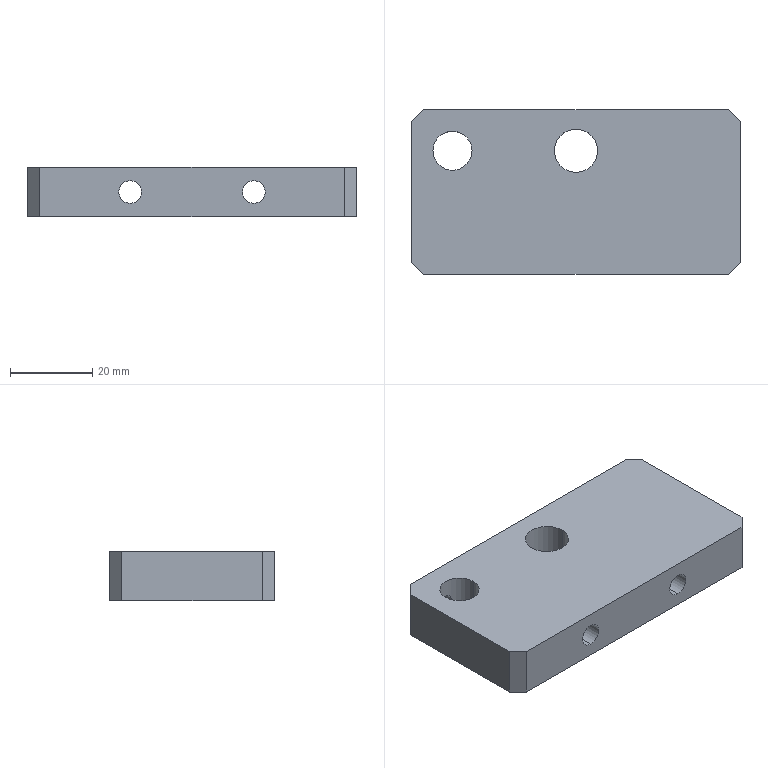Part | SolidWorks | features HoleWzd 2, Chamfer 1, Extrusion 1, ICE 1 | 1 solid | 26 faces | box 80 x 40 x 12 mm | volume 30513 mm3 | cylinder 14 | plane 12 | commonest cylinder face diameters 5.5 x4 10 x4 3.3 x2 9.5 x2 10.5 x2
STEP:
#1=CARTESIAN_POINT('',(-30.,14.75,4.35));
#2=VERTEX_POINT('',#1);
#3=CARTESIAN_POINT('',(-30.,14.75,7.65));
#4=VERTEX_POINT('',#3);
#5=CARTESIAN_POINT('',(-30.,14.75,4.35));
#6=CARTESIAN_POINT('',(-30.217,14.75,4.35));
#7=CARTESIAN_POINT('',(-30.435,14.734,4.394));
#8=CARTESIAN_POINT('',(-30.734,14.694,4.518));
#9=CARTESIAN_POINT('',(-30.83,14.678,4.57));
#10=CARTESIAN_POINT('',(-31.008,14.643,4.69));
#11=CARTESIAN_POINT('',(-31.091,14.624,4.757));
#12=CARTESIAN_POINT('',(-31.32,14.566,4.986));
#13=CARTESIAN_POINT('',(-31.44,14.527,5.166));
#14=CARTESIAN_POINT('',(-31.565,14.485,5.466));
#15=CARTESIAN_POINT('',(-31.597,14.474,5.569));
#16=CARTESIAN_POINT('',(-31.639,14.458,5.781));
#17=CARTESIAN_POINT('',(-31.65,14.454,5.892));
#18=CARTESIAN_POINT('',(-31.65,14.454,6.109));
#19=CARTESIAN_POINT('',(-31.639,14.458,6.217));
#20=CARTESIAN_POINT('',(-31.597,14.474,6.43));
#21=CARTESIAN_POINT('',(-31.564,14.485,6.535));
#22=CARTESIAN_POINT('',(-31.44,14.527,6.833));
#23=CARTESIAN_POINT('',(-31.318,14.566,7.015));
#24=CARTESIAN_POINT('',(-31.091,14.624,7.242));
#25=CARTESIAN_POINT('',(-31.007,14.643,7.312));
#26=CARTESIAN_POINT('',(-30.829,14.678,7.431));
#27=CARTESIAN_POINT('',(-30.734,14.694,7.481));
#28=CARTESIAN_POINT('',(-30.535,14.721,7.565));
#29=CARTESIAN_POINT('',(-30.43,14.732,7.597));
#30=CARTESIAN_POINT('',(-30.218,14.746,7.639));
#31=CARTESIAN_POINT('',(-30.11,14.75,7.65));
#32=CARTESIAN_POINT('',(-30.,14.75,7.65));
#33=B_SPLINE_CURVE_WITH_KNOTS('',3,(#5,#6,#7,#8,#9,#10,#11,#12,#13,#14,#15,#16,#17,#18,#19,#20,#21,#22,#23,#24,#25,#26,#27,#28,#29,#30,#31,#32),.UNSPECIFIED.,.F.,.F.,(4,2,2,2,2,2,2,2,2,2,2,2,2,4),(0.0052,0.005849,0.006174,0.006499,0.007149,0.007474,0.007799,0.008124,0.008448,0.009098,0.009423,0.009748,0.01007,0.0104),.UNSPECIFIED.);
#34=EDGE_CURVE('',#2,#4,#33,.T.);
#35=ORIENTED_EDGE('',*,*,#34,.F.);
#36=CARTESIAN_POINT('',(-30.,20.,4.35));
#37=VERTEX_POINT('',#36);
#38=CARTESIAN_POINT('',(-30.,20.,4.35));
#39=DIRECTION('',(0.,1.,0.));
#40=VECTOR('',#39,1000.);
#41=LINE('',#38,#40);
#42=EDGE_CURVE('',#2,#37,#41,.T.);
#43=ORIENTED_EDGE('',*,*,#42,.T.);
#44=CARTESIAN_POINT('',(-30.,20.,7.65));
#45=VERTEX_POINT('',#44);
#46=CARTESIAN_POINT('',(-30.,20.,6.));
#47=DIRECTION('',(0.,1.,0.));
#48=DIRECTION('',(0.,0.,1.));
#49=AXIS2_PLACEMENT_3D('',#46,#47,#48);
#50=CIRCLE('',#49,1.65);
#51=EDGE_CURVE('',#37,#45,#50,.T.);
#52=ORIENTED_EDGE('',*,*,#51,.T.);
#53=CARTESIAN_POINT('',(-30.,20.,7.65));
#54=DIRECTION('',(0.,1.,0.));
#55=VECTOR('',#54,1000.);
#56=LINE('',#53,#55);
#57=EDGE_CURVE('',#4,#45,#56,.T.);
#58=ORIENTED_EDGE('',*,*,#57,.F.);
#59=EDGE_LOOP('',(#35,#43,#52,#58));
#60=FACE_OUTER_BOUND('',#59,.T.);
#61=CARTESIAN_POINT('',(-30.,20.,6.));
#62=DIRECTION('',(0.,1.,0.));
#63=DIRECTION('',(0.,0.,1.));
#64=AXIS2_PLACEMENT_3D('',#61,#62,#63);
#65=CYLINDRICAL_SURFACE('',#64,1.65);
#66=ADVANCED_FACE('',(#60),#65,.F.);
#67=CARTESIAN_POINT('',(-15.,-15.,1.));
#68=VERTEX_POINT('',#67);
#69=CARTESIAN_POINT('',(-15.,-15.,11.));
#70=VERTEX_POINT('',#69);
#71=CARTESIAN_POINT('',(-15.,-15.,6.));
#72=DIRECTION('',(0.,1.,0.));
#73=DIRECTION('',(0.,0.,1.));
#74=AXIS2_PLACEMENT_3D('',#71,#72,#73);
#75=CIRCLE('',#74,5.);
#76=EDGE_CURVE('',#68,#70,#75,.T.);
#77=ORIENTED_EDGE('',*,*,#76,.F.);
#78=CARTESIAN_POINT('',(-15.,20.,1.));
#79=VERTEX_POINT('',#78);
#80=CARTESIAN_POINT('',(-15.,20.,1.));
#81=DIRECTION('',(0.,1.,0.));
#82=VECTOR('',#81,1000.);
#83=LINE('',#80,#82);
#84=EDGE_CURVE('',#68,#79,#83,.T.);
#85=ORIENTED_EDGE('',*,*,#84,.T.);
#86=CARTESIAN_POINT('',(-15.,20.,11.));
#87=VERTEX_POINT('',#86);
#88=CARTESIAN_POINT('',(-15.,20.,6.));
#89=DIRECTION('',(0.,1.,0.));
#90=DIRECTION('',(0.,0.,1.));
#91=AXIS2_PLACEMENT_3D('',#88,#89,#90);
#92=CIRCLE('',#91,5.);
#93=EDGE_CURVE('',#79,#87,#92,.T.);
#94=ORIENTED_EDGE('',*,*,#93,.T.);
#95=CARTESIAN_POINT('',(-15.,20.,11.));
#96=DIRECTION('',(0.,1.,0.));
#97=VECTOR('',#96,1000.);
#98=LINE('',#95,#97);
#99=EDGE_CURVE('',#70,#87,#98,.T.);
#100=ORIENTED_EDGE('',*,*,#99,.F.);
#101=EDGE_LOOP('',(#77,#85,#94,#100));
#102=FACE_OUTER_BOUND('',#101,.T.);
#103=CARTESIAN_POINT('',(-15.,20.,6.));
#104=DIRECTION('',(0.,1.,0.));
#105=DIRECTION('',(0.,0.,1.));
#106=AXIS2_PLACEMENT_3D('',#103,#104,#105);
#107=CYLINDRICAL_SURFACE('',#106,5.);
#108=ADVANCED_FACE('',(#102),#107,.F.);
#109=CARTESIAN_POINT('',(-15.,-20.,3.25));
#110=VERTEX_POINT('',#109);
#111=CARTESIAN_POINT('',(-15.,-20.,8.75));
#112=VERTEX_POINT('',#111);
#113=CARTESIAN_POINT('',(-15.,-20.,6.));
#114=DIRECTION('',(0.,1.,0.));
#115=DIRECTION('',(0.,0.,1.));
#116=AXIS2_PLACEMENT_3D('',#113,#114,#115);
#117=CIRCLE('',#116,2.75);
#118=EDGE_CURVE('',#110,#112,#117,.T.);
#119=ORIENTED_EDGE('',*,*,#118,.F.);
#120=CARTESIAN_POINT('',(-15.,-15.,3.25));
#121=VERTEX_POINT('',#120);
#122=CARTESIAN_POINT('',(-15.,20.,3.25));
#123=DIRECTION('',(0.,1.,0.));
#124=VECTOR('',#123,1000.);
#125=LINE('',#122,#124);
#126=EDGE_CURVE('',#110,#121,#125,.T.);
#127=ORIENTED_EDGE('',*,*,#126,.T.);
#128=CARTESIAN_POINT('',(-15.,-15.,8.75));
#129=VERTEX_POINT('',#128);
#130=CARTESIAN_POINT('',(-15.,-15.,6.));
#131=DIRECTION('',(0.,1.,0.));
#132=DIRECTION('',(0.,0.,1.));
#133=AXIS2_PLACEMENT_3D('',#130,#131,#132);
#134=CIRCLE('',#133,2.75);
#135=EDGE_CURVE('',#121,#129,#134,.T.);
#136=ORIENTED_EDGE('',*,*,#135,.T.);
#137=CARTESIAN_POINT('',(-15.,20.,8.75));
#138=DIRECTION('',(0.,1.,0.));
#139=VECTOR('',#138,1000.);
#140=LINE('',#137,#139);
#141=EDGE_CURVE('',#112,#129,#140,.T.);
#142=ORIENTED_EDGE('',*,*,#141,.F.);
#143=EDGE_LOOP('',(#119,#127,#136,#142));
#144=FACE_OUTER_BOUND('',#143,.T.);
#145=CARTESIAN_POINT('',(-15.,20.,6.));
#146=DIRECTION('',(0.,1.,0.));
#147=DIRECTION('',(0.,0.,1.));
#148=AXIS2_PLACEMENT_3D('',#145,#146,#147);
#149=CYLINDRICAL_SURFACE('',#148,2.75);
#150=ADVANCED_FACE('',(#144),#149,.F.);
#151=CARTESIAN_POINT('',(15.,-15.,1.));
#152=VERTEX_POINT('',#151);
#153=CARTESIAN_POINT('',(15.,-15.,11.));
#154=VERTEX_POINT('',#153);
#155=CARTESIAN_POINT('',(15.,-15.,6.));
#156=DIRECTION('',(0.,1.,0.));
#157=DIRECTION('',(0.,0.,1.));
#158=AXIS2_PLACEMENT_3D('',#155,#156,#157);
#159=CIRCLE('',#158,5.);
#160=EDGE_CURVE('',#152,#154,#159,.T.);
#161=ORIENTED_EDGE('',*,*,#160,.F.);
#162=CARTESIAN_POINT('',(15.,20.,1.));
#163=VERTEX_POINT('',#162);
#164=CARTESIAN_POINT('',(15.,20.,1.));
#165=DIRECTION('',(0.,1.,0.));
#166=VECTOR('',#165,1000.);
#167=LINE('',#164,#166);
#168=EDGE_CURVE('',#152,#163,#167,.T.);
#169=ORIENTED_EDGE('',*,*,#168,.T.);
#170=CARTESIAN_POINT('',(15.,20.,11.));
#171=VERTEX_POINT('',#170);
#172=CARTESIAN_POINT('',(15.,20.,6.));
#173=DIRECTION('',(0.,1.,0.));
#174=DIRECTION('',(0.,0.,1.));
#175=AXIS2_PLACEMENT_3D('',#172,#173,#174);
#176=CIRCLE('',#175,5.);
#177=EDGE_CURVE('',#163,#171,#176,.T.);
#178=ORIENTED_EDGE('',*,*,#177,.T.);
#179=CARTESIAN_POINT('',(15.,20.,11.));
#180=DIRECTION('',(0.,1.,0.));
#181=VECTOR('',#180,1000.);
#182=LINE('',#179,#181);
#183=EDGE_CURVE('',#154,#171,#182,.T.);
#184=ORIENTED_EDGE('',*,*,#183,.F.);
#185=EDGE_LOOP('',(#161,#169,#178,#184));
#186=FACE_OUTER_BOUND('',#185,.T.);
#187=CARTESIAN_POINT('',(15.,20.,6.));
#188=DIRECTION('',(0.,1.,0.));
#189=DIRECTION('',(0.,0.,1.));
#190=AXIS2_PLACEMENT_3D('',#187,#188,#189);
#191=CYLINDRICAL_SURFACE('',#190,5.);
#192=ADVANCED_FACE('',(#186),#191,.F.);
#193=CARTESIAN_POINT('',(15.,-20.,3.25));
#194=VERTEX_POINT('',#193);
#195=CARTESIAN_POINT('',(15.,-20.,8.75));
#196=VERTEX_POINT('',#195);
#197=CARTESIAN_POINT('',(15.,-20.,6.));
#198=DIRECTION('',(0.,1.,0.));
#199=DIRECTION('',(0.,0.,1.));
#200=AXIS2_PLACEMENT_3D('',#197,#198,#199);
#201=CIRCLE('',#200,2.75);
#202=EDGE_CURVE('',#194,#196,#201,.T.);
#203=ORIENTED_EDGE('',*,*,#202,.F.);
#204=CARTESIAN_POINT('',(15.,-15.,3.25));
#205=VERTEX_POINT('',#204);
#206=CARTESIAN_POINT('',(15.,20.,3.25));
#207=DIRECTION('',(0.,1.,0.));
#208=VECTOR('',#207,1000.);
#209=LINE('',#206,#208);
#210=EDGE_CURVE('',#194,#205,#209,.T.);
#211=ORIENTED_EDGE('',*,*,#210,.T.);
#212=CARTESIAN_POINT('',(15.,-15.,8.75));
#213=VERTEX_POINT('',#212);
#214=CARTESIAN_POINT('',(15.,-15.,6.));
#215=DIRECTION('',(0.,1.,0.));
#216=DIRECTION('',(0.,0.,1.));
#217=AXIS2_PLACEMENT_3D('',#214,#215,#216);
#218=CIRCLE('',#217,2.75);
#219=EDGE_CURVE('',#205,#213,#218,.T.);
#220=ORIENTED_EDGE('',*,*,#219,.T.);
#221=CARTESIAN_POINT('',(15.,20.,8.75));
#222=DIRECTION('',(0.,1.,0.));
#223=VECTOR('',#222,1000.);
#224=LINE('',#221,#223);
#225=EDGE_CURVE('',#196,#213,#224,.T.);
#226=ORIENTED_EDGE('',*,*,#225,.F.);
#227=EDGE_LOOP('',(#203,#211,#220,#226));
#228=FACE_OUTER_BOUND('',#227,.T.);
#229=CARTESIAN_POINT('',(15.,20.,6.));
#230=DIRECTION('',(0.,1.,0.));
#231=DIRECTION('',(0.,0.,1.));
#232=AXIS2_PLACEMENT_3D('',#229,#230,#231);
#233=CYLINDRICAL_SURFACE('',#232,2.75);
#234=ADVANCED_FACE('',(#228),#233,.F.);
#235=CARTESIAN_POINT('',(-34.75,10.,0.));
#236=VERTEX_POINT('',#235);
#237=CARTESIAN_POINT('',(-25.25,10.,0.));
#238=VERTEX_POINT('',#237);
#239=CARTESIAN_POINT('',(-30.,10.,0.));
#240=DIRECTION('',(0.,0.,1.));
#241=DIRECTION('',(1.,0.,0.));
#242=AXIS2_PLACEMENT_3D('',#239,#240,#241);
#243=CIRCLE('',#242,4.75);
#244=EDGE_CURVE('',#236,#238,#243,.T.);
#245=ORIENTED_EDGE('',*,*,#244,.F.);
#246=CARTESIAN_POINT('',(-34.75,10.,12.));
#247=VERTEX_POINT('',#246);
#248=CARTESIAN_POINT('',(-34.75,10.,0.));
#249=DIRECTION('',(0.,0.,1.));
#250=VECTOR('',#249,1000.);
#251=LINE('',#248,#250);
#252=EDGE_CURVE('',#236,#247,#251,.T.);
#253=ORIENTED_EDGE('',*,*,#252,.T.);
#254=CARTESIAN_POINT('',(-25.25,10.,12.));
#255=VERTEX_POINT('',#254);
#256=CARTESIAN_POINT('',(-30.,10.,12.));
#257=DIRECTION('',(0.,0.,1.));
#258=DIRECTION('',(1.,0.,0.));
#259=AXIS2_PLACEMENT_3D('',#256,#257,#258);
#260=CIRCLE('',#259,4.75);
#261=EDGE_CURVE('',#247,#255,#260,.T.);
#262=ORIENTED_EDGE('',*,*,#261,.T.);
#263=CARTESIAN_POINT('',(-25.25,10.,0.));
#264=DIRECTION('',(0.,0.,1.));
#265=VECTOR('',#264,1000.);
#266=LINE('',#263,#265);
#267=EDGE_CURVE('',#238,#255,#266,.T.);
#268=ORIENTED_EDGE('',*,*,#267,.F.);
#269=EDGE_LOOP('',(#245,#253,#262,#268));
#270=FACE_OUTER_BOUND('',#269,.T.);
#271=CARTESIAN_POINT('',(-30.,10.,0.));
#272=DIRECTION('',(0.,0.,1.));
#273=DIRECTION('',(1.,0.,0.));
#274=AXIS2_PLACEMENT_3D('',#271,#272,#273);
#275=CYLINDRICAL_SURFACE('',#274,4.75);
#276=ADVANCED_FACE('',(#270),#275,.F.);
#277=CARTESIAN_POINT('',(-5.25,10.,0.));
#278=VERTEX_POINT('',#277);
#279=CARTESIAN_POINT('',(5.25,10.,0.));
#280=VERTEX_POINT('',#279);
#281=CARTESIAN_POINT('',(0.,10.,0.));
#282=DIRECTION('',(0.,0.,1.));
#283=DIRECTION('',(1.,0.,0.));
#284=AXIS2_PLACEMENT_3D('',#281,#282,#283);
#285=CIRCLE('',#284,5.25);
#286=EDGE_CURVE('',#278,#280,#285,.T.);
#287=ORIENTED_EDGE('',*,*,#286,.F.);
#288=CARTESIAN_POINT('',(-5.25,10.,12.));
#289=VERTEX_POINT('',#288);
#290=CARTESIAN_POINT('',(-5.25,10.,0.));
#291=DIRECTION('',(0.,0.,1.));
#292=VECTOR('',#291,1000.);
#293=LINE('',#290,#292);
#294=EDGE_CURVE('',#278,#289,#293,.T.);
#295=ORIENTED_EDGE('',*,*,#294,.T.);
#296=CARTESIAN_POINT('',(5.25,10.,12.));
#297=VERTEX_POINT('',#296);
#298=CARTESIAN_POINT('',(0.,10.,12.));
#299=DIRECTION('',(0.,0.,1.));
#300=DIRECTION('',(1.,0.,0.));
#301=AXIS2_PLACEMENT_3D('',#298,#299,#300);
#302=CIRCLE('',#301,5.25);
#303=EDGE_CURVE('',#289,#297,#302,.T.);
#304=ORIENTED_EDGE('',*,*,#303,.T.);
#305=CARTESIAN_POINT('',(5.25,10.,0.));
#306=DIRECTION('',(0.,0.,1.));
#307=VECTOR('',#306,1000.);
#308=LINE('',#305,#307);
#309=EDGE_CURVE('',#280,#297,#308,.T.);
#310=ORIENTED_EDGE('',*,*,#309,.F.);
#311=EDGE_LOOP('',(#287,#295,#304,#310));
#312=FACE_OUTER_BOUND('',#311,.T.);
#313=CARTESIAN_POINT('',(0.,10.,0.));
#314=DIRECTION('',(0.,0.,1.));
#315=DIRECTION('',(1.,0.,0.));
#316=AXIS2_PLACEMENT_3D('',#313,#314,#315);
#317=CYLINDRICAL_SURFACE('',#316,5.25);
#318=ADVANCED_FACE('',(#312),#317,.F.);
#319=CARTESIAN_POINT('',(40.,-17.,12.));
#320=VERTEX_POINT('',#319);
#321=CARTESIAN_POINT('',(40.,17.,12.));
#322=VERTEX_POINT('',#321);
#323=CARTESIAN_POINT('',(40.,20.,12.));
#324=DIRECTION('',(0.,1.,0.));
#325=VECTOR('',#324,1000.);
#326=LINE('',#323,#325);
#327=EDGE_CURVE('',#320,#322,#326,.T.);
#328=ORIENTED_EDGE('',*,*,#327,.F.);
#329=CARTESIAN_POINT('',(40.,-17.,0.));
#330=VERTEX_POINT('',#329);
#331=CARTESIAN_POINT('',(40.,-17.,12.));
#332=DIRECTION('',(0.,0.,-1.));
#333=VECTOR('',#332,1000.);
#334=LINE('',#331,#333);
#335=EDGE_CURVE('',#320,#330,#334,.T.);
#336=ORIENTED_EDGE('',*,*,#335,.T.);
#337=CARTESIAN_POINT('',(40.,17.,0.));
#338=VERTEX_POINT('',#337);
#339=CARTESIAN_POINT('',(40.,20.,0.));
#340=DIRECTION('',(0.,1.,0.));
#341=VECTOR('',#340,1000.);
#342=LINE('',#339,#341);
#343=EDGE_CURVE('',#330,#338,#342,.T.);
#344=ORIENTED_EDGE('',*,*,#343,.T.);
#345=CARTESIAN_POINT('',(40.,17.,12.));
#346=DIRECTION('',(0.,0.,1.));
#347=VECTOR('',#346,1000.);
#348=LINE('',#345,#347);
#349=EDGE_CURVE('',#338,#322,#348,.T.);
#350=ORIENTED_EDGE('',*,*,#349,.T.);
#351=EDGE_LOOP('',(#328,#336,#344,#350));
#352=FACE_OUTER_BOUND('',#351,.T.);
#353=CARTESIAN_POINT('',(40.,20.,12.));
#354=DIRECTION('',(-1.,0.,0.));
#355=DIRECTION('',(0.,0.,1.));
#356=AXIS2_PLACEMENT_3D('',#353,#354,#355);
#357=PLANE('',#356);
#358=ADVANCED_FACE('',(#352),#357,.F.);
#359=CARTESIAN_POINT('',(-30.,20.,6.));
#360=DIRECTION('',(0.,1.,0.));
#361=DIRECTION('',(0.,0.,1.));
#362=AXIS2_PLACEMENT_3D('',#359,#360,#361);
#363=CIRCLE('',#362,1.65);
#364=EDGE_CURVE('',#45,#37,#363,.T.);
#365=ORIENTED_EDGE('',*,*,#364,.F.);
#366=ORIENTED_EDGE('',*,*,#51,.F.);
#367=EDGE_LOOP('',(#365,#366));
#368=FACE_BOUND('',#367,.T.);
#369=CARTESIAN_POINT('',(-15.,20.,6.));
#370=DIRECTION('',(0.,1.,0.));
#371=DIRECTION('',(0.,0.,1.));
#372=AXIS2_PLACEMENT_3D('',#369,#370,#371);
#373=CIRCLE('',#372,5.);
#374=EDGE_CURVE('',#87,#79,#373,.T.);
#375=ORIENTED_EDGE('',*,*,#374,.F.);
#376=ORIENTED_EDGE('',*,*,#93,.F.);
#377=EDGE_LOOP('',(#375,#376));
#378=FACE_BOUND('',#377,.T.);
#379=CARTESIAN_POINT('',(15.,20.,6.));
#380=DIRECTION('',(0.,1.,0.));
#381=DIRECTION('',(0.,0.,1.));
#382=AXIS2_PLACEMENT_3D('',#379,#380,#381);
#383=CIRCLE('',#382,5.);
#384=EDGE_CURVE('',#171,#163,#383,.T.);
#385=ORIENTED_EDGE('',*,*,#384,.F.);
#386=ORIENTED_EDGE('',*,*,#177,.F.);
#387=EDGE_LOOP('',(#385,#386));
#388=FACE_BOUND('',#387,.T.);
#389=CARTESIAN_POINT('',(37.,20.,12.));
#390=VERTEX_POINT('',#389);
#391=CARTESIAN_POINT('',(-37.,20.,12.));
#392=VERTEX_POINT('',#391);
#393=CARTESIAN_POINT('',(-40.,20.,12.));
#394=DIRECTION('',(-1.,0.,0.));
#395=VECTOR('',#394,1000.);
#396=LINE('',#393,#395);
#397=EDGE_CURVE('',#390,#392,#396,.T.);
#398=ORIENTED_EDGE('',*,*,#397,.F.);
#399=CARTESIAN_POINT('',(37.,20.,0.));
#400=VERTEX_POINT('',#399);
#401=CARTESIAN_POINT('',(37.,20.,12.));
#402=DIRECTION('',(0.,0.,-1.));
#403=VECTOR('',#402,1000.);
#404=LINE('',#401,#403);
#405=EDGE_CURVE('',#390,#400,#404,.T.);
#406=ORIENTED_EDGE('',*,*,#405,.T.);
#407=CARTESIAN_POINT('',(-37.,20.,0.));
#408=VERTEX_POINT('',#407);
#409=CARTESIAN_POINT('',(-40.,20.,0.));
#410=DIRECTION('',(-1.,0.,0.));
#411=VECTOR('',#410,1000.);
#412=LINE('',#409,#411);
#413=EDGE_CURVE('',#400,#408,#412,.T.);
#414=ORIENTED_EDGE('',*,*,#413,.T.);
#415=CARTESIAN_POINT('',(-37.,20.,12.));
#416=DIRECTION('',(0.,0.,1.));
#417=VECTOR('',#416,1000.);
#418=LINE('',#415,#417);
#419=EDGE_CURVE('',#408,#392,#418,.T.);
#420=ORIENTED_EDGE('',*,*,#419,.T.);
#421=EDGE_LOOP('',(#398,#406,#414,#420));
#422=FACE_OUTER_BOUND('',#421,.T.);
#423=CARTESIAN_POINT('',(-40.,20.,12.));
#424=DIRECTION('',(0.,-1.,0.));
#425=DIRECTION('',(0.,0.,-1.));
#426=AXIS2_PLACEMENT_3D('',#423,#424,#425);
#427=PLANE('',#426);
#428=ADVANCED_FACE('',(#368,#378,#388,#422),#427,.F.);
#429=CARTESIAN_POINT('',(-40.,17.,0.));
#430=VERTEX_POINT('',#429);
#431=CARTESIAN_POINT('',(-40.,-17.,0.));
#432=VERTEX_POINT('',#431);
#433=CARTESIAN_POINT('',(-40.,20.,0.));
#434=DIRECTION('',(0.,-1.,0.));
#435=VECTOR('',#434,1000.);
#436=LINE('',#433,#435);
#437=EDGE_CURVE('',#430,#432,#436,.T.);
#438=ORIENTED_EDGE('',*,*,#437,.T.);
#439=CARTESIAN_POINT('',(-40.,-17.,12.));
#440=VERTEX_POINT('',#439);
#441=CARTESIAN_POINT('',(-40.,-17.,12.));
#442=DIRECTION('',(0.,0.,1.));
#443=VECTOR('',#442,1000.);
#444=LINE('',#441,#443);
#445=EDGE_CURVE('',#432,#440,#444,.T.);
#446=ORIENTED_EDGE('',*,*,#445,.T.);
#447=CARTESIAN_POINT('',(-40.,17.,12.));
#448=VERTEX_POINT('',#447);
#449=CARTESIAN_POINT('',(-40.,20.,12.));
#450=DIRECTION('',(0.,-1.,0.));
#451=VECTOR('',#450,1000.);
#452=LINE('',#449,#451);
#453=EDGE_CURVE('',#448,#440,#452,.T.);
#454=ORIENTED_EDGE('',*,*,#453,.F.);
#455=CARTESIAN_POINT('',(-40.,17.,12.));
#456=DIRECTION('',(0.,0.,-1.));
#457=VECTOR('',#456,1000.);
#458=LINE('',#455,#457);
#459=EDGE_CURVE('',#448,#430,#458,.T.);
#460=ORIENTED_EDGE('',*,*,#459,.T.);
#461=EDGE_LOOP('',(#438,#446,#454,#460));
#462=FACE_OUTER_BOUND('',#461,.T.);
#463=CARTESIAN_POINT('',(-40.,20.,12.));
#464=DIRECTION('',(1.,0.,0.));
#465=DIRECTION('',(0.,1.,0.));
#466=AXIS2_PLACEMENT_3D('',#463,#464,#465);
#467=PLANE('',#466);
#468=ADVANCED_FACE('',(#462),#467,.F.);
#469=CARTESIAN_POINT('',(-15.,-20.,6.));
#470=DIRECTION('',(0.,1.,0.));
#471=DIRECTION('',(0.,0.,1.));
#472=AXIS2_PLACEMENT_3D('',#469,#470,#471);
#473=CIRCLE('',#472,2.75);
#474=EDGE_CURVE('',#112,#110,#473,.T.);
#475=ORIENTED_EDGE('',*,*,#474,.T.);
#476=ORIENTED_EDGE('',*,*,#118,.T.);
#477=EDGE_LOOP('',(#475,#476));
#478=FACE_BOUND('',#477,.T.);
#479=CARTESIAN_POINT('',(15.,-20.,6.));
#480=DIRECTION('',(0.,1.,0.));
#481=DIRECTION('',(0.,0.,1.));
#482=AXIS2_PLACEMENT_3D('',#479,#480,#481);
#483=CIRCLE('',#482,2.75);
#484=EDGE_CURVE('',#196,#194,#483,.T.);
#485=ORIENTED_EDGE('',*,*,#484,.T.);
#486=ORIENTED_EDGE('',*,*,#202,.T.);
#487=EDGE_LOOP('',(#485,#486));
#488=FACE_BOUND('',#487,.T.);
#489=CARTESIAN_POINT('',(-37.,-20.,12.));
#490=VERTEX_POINT('',#489);
#491=CARTESIAN_POINT('',(37.,-20.,12.));
#492=VERTEX_POINT('',#491);
#493=CARTESIAN_POINT('',(-40.,-20.,12.));
#494=DIRECTION('',(1.,0.,0.));
#495=VECTOR('',#494,1000.);
#496=LINE('',#493,#495);
#497=EDGE_CURVE('',#490,#492,#496,.T.);
#498=ORIENTED_EDGE('',*,*,#497,.F.);
#499=CARTESIAN_POINT('',(-37.,-20.,0.));
#500=VERTEX_POINT('',#499);
#501=CARTESIAN_POINT('',(-37.,-20.,12.));
#502=DIRECTION('',(0.,0.,-1.));
#503=VECTOR('',#502,1000.);
#504=LINE('',#501,#503);
#505=EDGE_CURVE('',#490,#500,#504,.T.);
#506=ORIENTED_EDGE('',*,*,#505,.T.);
#507=CARTESIAN_POINT('',(37.,-20.,0.));
#508=VERTEX_POINT('',#507);
#509=CARTESIAN_POINT('',(-40.,-20.,0.));
#510=DIRECTION('',(1.,0.,0.));
#511=VECTOR('',#510,1000.);
#512=LINE('',#509,#511);
#513=EDGE_CURVE('',#500,#508,#512,.T.);
#514=ORIENTED_EDGE('',*,*,#513,.T.);
#515=CARTESIAN_POINT('',(37.,-20.,12.));
#516=DIRECTION('',(0.,0.,1.));
#517=VECTOR('',#516,1000.);
#518=LINE('',#515,#517);
#519=EDGE_CURVE('',#508,#492,#518,.T.);
#520=ORIENTED_EDGE('',*,*,#519,.T.);
#521=EDGE_LOOP('',(#498,#506,#514,#520));
#522=FACE_OUTER_BOUND('',#521,.T.);
#523=CARTESIAN_POINT('',(-40.,-20.,12.));
#524=DIRECTION('',(0.,1.,0.));
#525=DIRECTION('',(0.,0.,1.));
#526=AXIS2_PLACEMENT_3D('',#523,#524,#525);
#527=PLANE('',#526);
#528=ADVANCED_FACE('',(#478,#488,#522),#527,.F.);
#529=CARTESIAN_POINT('',(-30.,10.,12.));
#530=DIRECTION('',(0.,0.,1.));
#531=DIRECTION('',(1.,0.,0.));
#532=AXIS2_PLACEMENT_3D('',#529,#530,#531);
#533=CIRCLE('',#532,4.75);
#534=EDGE_CURVE('',#255,#247,#533,.T.);
#535=ORIENTED_EDGE('',*,*,#534,.F.);
#536=ORIENTED_EDGE('',*,*,#261,.F.);
#537=EDGE_LOOP('',(#535,#536));
#538=FACE_BOUND('',#537,.T.);
#539=CARTESIAN_POINT('',(0.,10.,12.));
#540=DIRECTION('',(0.,0.,1.));
#541=DIRECTION('',(1.,0.,0.));
#542=AXIS2_PLACEMENT_3D('',#539,#540,#541);
#543=CIRCLE('',#542,5.25);
#544=EDGE_CURVE('',#297,#289,#543,.T.);
#545=ORIENTED_EDGE('',*,*,#544,.F.);
#546=ORIENTED_EDGE('',*,*,#303,.F.);
#547=EDGE_LOOP('',(#545,#546));
#548=FACE_BOUND('',#547,.T.);
#549=ORIENTED_EDGE('',*,*,#453,.T.);
#550=CARTESIAN_POINT('',(-28.5,-28.5,12.));
#551=DIRECTION('',(0.7071,-0.7071,0.));
#552=VECTOR('',#551,1000.);
#553=LINE('',#550,#552);
#554=EDGE_CURVE('',#440,#490,#553,.T.);
#555=ORIENTED_EDGE('',*,*,#554,.T.);
#556=ORIENTED_EDGE('',*,*,#497,.T.);
#557=CARTESIAN_POINT('',(28.5,-28.5,12.));
#558=DIRECTION('',(0.7071,0.7071,0.));
#559=VECTOR('',#558,1000.);
#560=LINE('',#557,#559);
#561=EDGE_CURVE('',#492,#320,#560,.T.);
#562=ORIENTED_EDGE('',*,*,#561,.T.);
#563=ORIENTED_EDGE('',*,*,#327,.T.);
#564=CARTESIAN_POINT('',(28.5,28.5,12.));
#565=DIRECTION('',(-0.7071,0.7071,0.));
#566=VECTOR('',#565,1000.);
#567=LINE('',#564,#566);
#568=EDGE_CURVE('',#322,#390,#567,.T.);
#569=ORIENTED_EDGE('',*,*,#568,.T.);
#570=ORIENTED_EDGE('',*,*,#397,.T.);
#571=CARTESIAN_POINT('',(-28.5,28.5,12.));
#572=DIRECTION('',(-0.7071,-0.7071,0.));
#573=VECTOR('',#572,1000.);
#574=LINE('',#571,#573);
#575=EDGE_CURVE('',#392,#448,#574,.T.);
#576=ORIENTED_EDGE('',*,*,#575,.T.);
#577=EDGE_LOOP('',(#549,#555,#556,#562,#563,#569,#570,#576));
#578=FACE_OUTER_BOUND('',#577,.T.);
#579=CARTESIAN_POINT('',(0.,0.,12.));
#580=DIRECTION('',(0.,0.,1.));
#581=DIRECTION('',(1.,0.,0.));
#582=AXIS2_PLACEMENT_3D('',#579,#580,#581);
#583=PLANE('',#582);
#584=ADVANCED_FACE('',(#538,#548,#578),#583,.T.);
#585=CARTESIAN_POINT('',(-30.,10.,0.));
#586=DIRECTION('',(0.,0.,1.));
#587=DIRECTION('',(1.,0.,0.));
#588=AXIS2_PLACEMENT_3D('',#585,#586,#587);
#589=CIRCLE('',#588,4.75);
#590=EDGE_CURVE('',#238,#236,#589,.T.);
#591=ORIENTED_EDGE('',*,*,#590,.T.);
#592=ORIENTED_EDGE('',*,*,#244,.T.);
#593=EDGE_LOOP('',(#591,#592));
#594=FACE_BOUND('',#593,.T.);
#595=CARTESIAN_POINT('',(0.,10.,0.));
#596=DIRECTION('',(0.,0.,1.));
#597=DIRECTION('',(1.,0.,0.));
#598=AXIS2_PLACEMENT_3D('',#595,#596,#597);
#599=CIRCLE('',#598,5.25);
#600=EDGE_CURVE('',#280,#278,#599,.T.);
#601=ORIENTED_EDGE('',*,*,#600,.T.);
#602=ORIENTED_EDGE('',*,*,#286,.T.);
#603=EDGE_LOOP('',(#601,#602));
#604=FACE_BOUND('',#603,.T.);
#605=ORIENTED_EDGE('',*,*,#513,.F.);
#606=CARTESIAN_POINT('',(-37.,-20.,0.));
#607=DIRECTION('',(-0.7071,0.7071,0.));
#608=VECTOR('',#607,1000.);
#609=LINE('',#606,#608);
#610=EDGE_CURVE('',#500,#432,#609,.T.);
#611=ORIENTED_EDGE('',*,*,#610,.T.);
#612=ORIENTED_EDGE('',*,*,#437,.F.);
#613=CARTESIAN_POINT('',(-40.,17.,0.));
#614=DIRECTION('',(0.7071,0.7071,0.));
#615=VECTOR('',#614,1000.);
#616=LINE('',#613,#615);
#617=EDGE_CURVE('',#430,#408,#616,.T.);
#618=ORIENTED_EDGE('',*,*,#617,.T.);
#619=ORIENTED_EDGE('',*,*,#413,.F.);
#620=CARTESIAN_POINT('',(37.,20.,0.));
#621=DIRECTION('',(0.7071,-0.7071,0.));
#622=VECTOR('',#621,1000.);
#623=LINE('',#620,#622);
#624=EDGE_CURVE('',#400,#338,#623,.T.);
#625=ORIENTED_EDGE('',*,*,#624,.T.);
#626=ORIENTED_EDGE('',*,*,#343,.F.);
#627=CARTESIAN_POINT('',(40.,-17.,0.));
#628=DIRECTION('',(-0.7071,-0.7071,0.));
#629=VECTOR('',#628,1000.);
#630=LINE('',#627,#629);
#631=EDGE_CURVE('',#330,#508,#630,.T.);
#632=ORIENTED_EDGE('',*,*,#631,.T.);
#633=EDGE_LOOP('',(#605,#611,#612,#618,#619,#625,#626,#632));
#634=FACE_OUTER_BOUND('',#633,.T.);
#635=CARTESIAN_POINT('',(0.,0.,0.));
#636=DIRECTION('',(0.,0.,1.));
#637=DIRECTION('',(1.,0.,0.));
#638=AXIS2_PLACEMENT_3D('',#635,#636,#637);
#639=PLANE('',#638);
#640=ADVANCED_FACE('',(#594,#604,#634),#639,.F.);
#641=ORIENTED_EDGE('',*,*,#294,.F.);
#642=ORIENTED_EDGE('',*,*,#600,.F.);
#643=ORIENTED_EDGE('',*,*,#309,.T.);
#644=ORIENTED_EDGE('',*,*,#544,.T.);
#645=EDGE_LOOP('',(#641,#642,#643,#644));
#646=FACE_OUTER_BOUND('',#645,.T.);
#647=CARTESIAN_POINT('',(0.,10.,0.));
#648=DIRECTION('',(0.,0.,1.));
#649=DIRECTION('',(1.,0.,0.));
#650=AXIS2_PLACEMENT_3D('',#647,#648,#649);
#651=CYLINDRICAL_SURFACE('',#650,5.25);
#652=ADVANCED_FACE('',(#646),#651,.F.);
#653=ORIENTED_EDGE('',*,*,#252,.F.);
#654=ORIENTED_EDGE('',*,*,#590,.F.);
#655=ORIENTED_EDGE('',*,*,#267,.T.);
#656=ORIENTED_EDGE('',*,*,#534,.T.);
#657=EDGE_LOOP('',(#653,#654,#655,#656));
#658=FACE_OUTER_BOUND('',#657,.T.);
#659=CARTESIAN_POINT('',(-30.,14.75,7.65));
#660=CARTESIAN_POINT('',(-29.89,14.75,7.65));
#661=CARTESIAN_POINT('',(-29.782,14.746,7.639));
#662=CARTESIAN_POINT('',(-29.57,14.732,7.597));
#663=CARTESIAN_POINT('',(-29.465,14.721,7.565));
#664=CARTESIAN_POINT('',(-29.265,14.694,7.481));
#665=CARTESIAN_POINT('',(-29.171,14.678,7.431));
#666=CARTESIAN_POINT('',(-28.992,14.643,7.311));
#667=CARTESIAN_POINT('',(-28.908,14.623,7.242));
#668=CARTESIAN_POINT('',(-28.682,14.566,7.015));
#669=CARTESIAN_POINT('',(-28.559,14.527,6.833));
#670=CARTESIAN_POINT('',(-28.436,14.485,6.535));
#671=CARTESIAN_POINT('',(-28.403,14.474,6.43));
#672=CARTESIAN_POINT('',(-28.361,14.458,6.217));
#673=CARTESIAN_POINT('',(-28.35,14.454,6.109));
#674=CARTESIAN_POINT('',(-28.35,14.454,5.892));
#675=CARTESIAN_POINT('',(-28.361,14.458,5.782));
#676=CARTESIAN_POINT('',(-28.403,14.474,5.57));
#677=CARTESIAN_POINT('',(-28.435,14.485,5.466));
#678=CARTESIAN_POINT('',(-28.56,14.527,5.165));
#679=CARTESIAN_POINT('',(-28.682,14.566,4.984));
#680=CARTESIAN_POINT('',(-28.91,14.624,4.757));
#681=CARTESIAN_POINT('',(-28.992,14.643,4.689));
#682=CARTESIAN_POINT('',(-29.17,14.678,4.57));
#683=CARTESIAN_POINT('',(-29.267,14.694,4.518));
#684=CARTESIAN_POINT('',(-29.565,14.734,4.394));
#685=CARTESIAN_POINT('',(-29.783,14.75,4.35));
#686=CARTESIAN_POINT('',(-30.,14.75,4.35));
#687=B_SPLINE_CURVE_WITH_KNOTS('',3,(#659,#660,#661,#662,#663,#664,#665,#666,#667,#668,#669,#670,#671,#672,#673,#674,#675,#676,#677,#678,#679,#680,#681,#682,#683,#684,#685,#686),.UNSPECIFIED.,.F.,.F.,(4,2,2,2,2,2,2,2,2,2,2,2,2,4),(0.,0.000325,0.0006499,0.0009749,0.0013,0.00195,0.002275,0.0026,0.002925,0.00325,0.0039,0.004225,0.00455,0.0052),.UNSPECIFIED.);
#688=EDGE_CURVE('',#4,#2,#687,.T.);
#689=ORIENTED_EDGE('',*,*,#688,.T.);
#690=ORIENTED_EDGE('',*,*,#34,.T.);
#691=EDGE_LOOP('',(#689,#690));
#692=FACE_BOUND('',#691,.T.);
#693=CARTESIAN_POINT('',(-30.,10.,0.));
#694=DIRECTION('',(0.,0.,1.));
#695=DIRECTION('',(1.,0.,0.));
#696=AXIS2_PLACEMENT_3D('',#693,#694,#695);
#697=CYLINDRICAL_SURFACE('',#696,4.75);
#698=ADVANCED_FACE('',(#658,#692),#697,.F.);
#699=ORIENTED_EDGE('',*,*,#210,.F.);
#700=ORIENTED_EDGE('',*,*,#484,.F.);
#701=ORIENTED_EDGE('',*,*,#225,.T.);
#702=CARTESIAN_POINT('',(15.,-15.,6.));
#703=DIRECTION('',(0.,1.,0.));
#704=DIRECTION('',(0.,0.,1.));
#705=AXIS2_PLACEMENT_3D('',#702,#703,#704);
#706=CIRCLE('',#705,2.75);
#707=EDGE_CURVE('',#213,#205,#706,.T.);
#708=ORIENTED_EDGE('',*,*,#707,.T.);
#709=EDGE_LOOP('',(#699,#700,#701,#708));
#710=FACE_OUTER_BOUND('',#709,.T.);
#711=CARTESIAN_POINT('',(15.,20.,6.));
#712=DIRECTION('',(0.,1.,0.));
#713=DIRECTION('',(0.,0.,1.));
#714=AXIS2_PLACEMENT_3D('',#711,#712,#713);
#715=CYLINDRICAL_SURFACE('',#714,2.75);
#716=ADVANCED_FACE('',(#710),#715,.F.);
#717=ORIENTED_EDGE('',*,*,#707,.F.);
#718=ORIENTED_EDGE('',*,*,#219,.F.);
#719=EDGE_LOOP('',(#717,#718));
#720=FACE_BOUND('',#719,.T.);
#721=CARTESIAN_POINT('',(15.,-15.,6.));
#722=DIRECTION('',(0.,1.,0.));
#723=DIRECTION('',(0.,0.,1.));
#724=AXIS2_PLACEMENT_3D('',#721,#722,#723);
#725=CIRCLE('',#724,5.);
#726=EDGE_CURVE('',#154,#152,#725,.T.);
#727=ORIENTED_EDGE('',*,*,#726,.T.);
#728=ORIENTED_EDGE('',*,*,#160,.T.);
#729=EDGE_LOOP('',(#727,#728));
#730=FACE_OUTER_BOUND('',#729,.T.);
#731=CARTESIAN_POINT('',(17.75,-15.,6.));
#732=DIRECTION('',(0.,-1.,0.));
#733=DIRECTION('',(0.,0.,-1.));
#734=AXIS2_PLACEMENT_3D('',#731,#732,#733);
#735=PLANE('',#734);
#736=ADVANCED_FACE('',(#720,#730),#735,.F.);
#737=ORIENTED_EDGE('',*,*,#168,.F.);
#738=ORIENTED_EDGE('',*,*,#726,.F.);
#739=ORIENTED_EDGE('',*,*,#183,.T.);
#740=ORIENTED_EDGE('',*,*,#384,.T.);
#741=EDGE_LOOP('',(#737,#738,#739,#740));
#742=FACE_OUTER_BOUND('',#741,.T.);
#743=CARTESIAN_POINT('',(15.,20.,6.));
#744=DIRECTION('',(0.,1.,0.));
#745=DIRECTION('',(0.,0.,1.));
#746=AXIS2_PLACEMENT_3D('',#743,#744,#745);
#747=CYLINDRICAL_SURFACE('',#746,5.);
#748=ADVANCED_FACE('',(#742),#747,.F.);
#749=ORIENTED_EDGE('',*,*,#126,.F.);
#750=ORIENTED_EDGE('',*,*,#474,.F.);
#751=ORIENTED_EDGE('',*,*,#141,.T.);
#752=CARTESIAN_POINT('',(-15.,-15.,6.));
#753=DIRECTION('',(0.,1.,0.));
#754=DIRECTION('',(0.,0.,1.));
#755=AXIS2_PLACEMENT_3D('',#752,#753,#754);
#756=CIRCLE('',#755,2.75);
#757=EDGE_CURVE('',#129,#121,#756,.T.);
#758=ORIENTED_EDGE('',*,*,#757,.T.);
#759=EDGE_LOOP('',(#749,#750,#751,#758));
#760=FACE_OUTER_BOUND('',#759,.T.);
#761=CARTESIAN_POINT('',(-15.,20.,6.));
#762=DIRECTION('',(0.,1.,0.));
#763=DIRECTION('',(0.,0.,1.));
#764=AXIS2_PLACEMENT_3D('',#761,#762,#763);
#765=CYLINDRICAL_SURFACE('',#764,2.75);
#766=ADVANCED_FACE('',(#760),#765,.F.);
#767=ORIENTED_EDGE('',*,*,#757,.F.);
#768=ORIENTED_EDGE('',*,*,#135,.F.);
#769=EDGE_LOOP('',(#767,#768));
#770=FACE_BOUND('',#769,.T.);
#771=CARTESIAN_POINT('',(-15.,-15.,6.));
#772=DIRECTION('',(0.,1.,0.));
#773=DIRECTION('',(0.,0.,1.));
#774=AXIS2_PLACEMENT_3D('',#771,#772,#773);
#775=CIRCLE('',#774,5.);
#776=EDGE_CURVE('',#70,#68,#775,.T.);
#777=ORIENTED_EDGE('',*,*,#776,.T.);
#778=ORIENTED_EDGE('',*,*,#76,.T.);
#779=EDGE_LOOP('',(#777,#778));
#780=FACE_OUTER_BOUND('',#779,.T.);
#781=CARTESIAN_POINT('',(-12.25,-15.,6.));
#782=DIRECTION('',(0.,-1.,0.));
#783=DIRECTION('',(0.,0.,-1.));
#784=AXIS2_PLACEMENT_3D('',#781,#782,#783);
#785=PLANE('',#784);
#786=ADVANCED_FACE('',(#770,#780),#785,.F.);
#787=ORIENTED_EDGE('',*,*,#84,.F.);
#788=ORIENTED_EDGE('',*,*,#776,.F.);
#789=ORIENTED_EDGE('',*,*,#99,.T.);
#790=ORIENTED_EDGE('',*,*,#374,.T.);
#791=EDGE_LOOP('',(#787,#788,#789,#790));
#792=FACE_OUTER_BOUND('',#791,.T.);
#793=CARTESIAN_POINT('',(-15.,20.,6.));
#794=DIRECTION('',(0.,1.,0.));
#795=DIRECTION('',(0.,0.,1.));
#796=AXIS2_PLACEMENT_3D('',#793,#794,#795);
#797=CYLINDRICAL_SURFACE('',#796,5.);
#798=ADVANCED_FACE('',(#792),#797,.F.);
#799=ORIENTED_EDGE('',*,*,#554,.F.);
#800=ORIENTED_EDGE('',*,*,#445,.F.);
#801=ORIENTED_EDGE('',*,*,#610,.F.);
#802=ORIENTED_EDGE('',*,*,#505,.F.);
#803=EDGE_LOOP('',(#799,#800,#801,#802));
#804=FACE_OUTER_BOUND('',#803,.T.);
#805=CARTESIAN_POINT('',(-37.,-20.,12.));
#806=DIRECTION('',(0.7071,0.7071,0.));
#807=DIRECTION('',(0.,0.,-1.));
#808=AXIS2_PLACEMENT_3D('',#805,#806,#807);
#809=PLANE('',#808);
#810=ADVANCED_FACE('',(#804),#809,.F.);
#811=ORIENTED_EDGE('',*,*,#561,.F.);
#812=ORIENTED_EDGE('',*,*,#519,.F.);
#813=ORIENTED_EDGE('',*,*,#631,.F.);
#814=ORIENTED_EDGE('',*,*,#335,.F.);
#815=EDGE_LOOP('',(#811,#812,#813,#814));
#816=FACE_OUTER_BOUND('',#815,.T.);
#817=CARTESIAN_POINT('',(40.,-17.,12.));
#818=DIRECTION('',(-0.7071,0.7071,0.));
#819=DIRECTION('',(0.,0.,-1.));
#820=AXIS2_PLACEMENT_3D('',#817,#818,#819);
#821=PLANE('',#820);
#822=ADVANCED_FACE('',(#816),#821,.F.);
#823=ORIENTED_EDGE('',*,*,#568,.F.);
#824=ORIENTED_EDGE('',*,*,#349,.F.);
#825=ORIENTED_EDGE('',*,*,#624,.F.);
#826=ORIENTED_EDGE('',*,*,#405,.F.);
#827=EDGE_LOOP('',(#823,#824,#825,#826));
#828=FACE_OUTER_BOUND('',#827,.T.);
#829=CARTESIAN_POINT('',(37.,20.,12.));
#830=DIRECTION('',(-0.7071,-0.7071,0.));
#831=DIRECTION('',(0.,0.,-1.));
#832=AXIS2_PLACEMENT_3D('',#829,#830,#831);
#833=PLANE('',#832);
#834=ADVANCED_FACE('',(#828),#833,.F.);
#835=ORIENTED_EDGE('',*,*,#575,.F.);
#836=ORIENTED_EDGE('',*,*,#419,.F.);
#837=ORIENTED_EDGE('',*,*,#617,.F.);
#838=ORIENTED_EDGE('',*,*,#459,.F.);
#839=EDGE_LOOP('',(#835,#836,#837,#838));
#840=FACE_OUTER_BOUND('',#839,.T.);
#841=CARTESIAN_POINT('',(-40.,17.,12.));
#842=DIRECTION('',(0.7071,-0.7071,0.));
#843=DIRECTION('',(0.,0.,-1.));
#844=AXIS2_PLACEMENT_3D('',#841,#842,#843);
#845=PLANE('',#844);
#846=ADVANCED_FACE('',(#840),#845,.F.);
#847=ORIENTED_EDGE('',*,*,#42,.F.);
#848=ORIENTED_EDGE('',*,*,#688,.F.);
#849=ORIENTED_EDGE('',*,*,#57,.T.);
#850=ORIENTED_EDGE('',*,*,#364,.T.);
#851=EDGE_LOOP('',(#847,#848,#849,#850));
#852=FACE_OUTER_BOUND('',#851,.T.);
#853=CARTESIAN_POINT('',(-30.,20.,6.));
#854=DIRECTION('',(0.,1.,0.));
#855=DIRECTION('',(0.,0.,1.));
#856=AXIS2_PLACEMENT_3D('',#853,#854,#855);
#857=CYLINDRICAL_SURFACE('',#856,1.65);
#858=ADVANCED_FACE('',(#852),#857,.F.);
#859=CLOSED_SHELL('',(#66,#108,#150,#192,#234,#276,#318,#358,#428,#468,#528,#584,#640,#652,#698,#716,#736,#748,#766,#786,#798,#810,#822,#834,#846,#858));
#860=MANIFOLD_SOLID_BREP('',#859);
#861=CARTESIAN_POINT('',(0.,0.,0.));
#862=DIRECTION('',(0.,0.,1.));
#863=DIRECTION('',(1.,0.,0.));
#864=AXIS2_PLACEMENT_3D('',#861,#862,#863);
#865=(LENGTH_UNIT()NAMED_UNIT(*)SI_UNIT(.MILLI.,.METRE.));
#866=UNCERTAINTY_MEASURE_WITH_UNIT(LENGTH_MEASURE(0.00001),#865,'','');
#867=(NAMED_UNIT(*)PLANE_ANGLE_UNIT()SI_UNIT($,.RADIAN.));
#868=(NAMED_UNIT(*)SI_UNIT($,.STERADIAN.)SOLID_ANGLE_UNIT());
#869=(GEOMETRIC_REPRESENTATION_CONTEXT(3)GLOBAL_UNCERTAINTY_ASSIGNED_CONTEXT((#866))GLOBAL_UNIT_ASSIGNED_CONTEXT((#865,#867,#868))REPRESENTATION_CONTEXT('',''));
#870=ADVANCED_BREP_SHAPE_REPRESENTATION('',(#860,#864),#869);